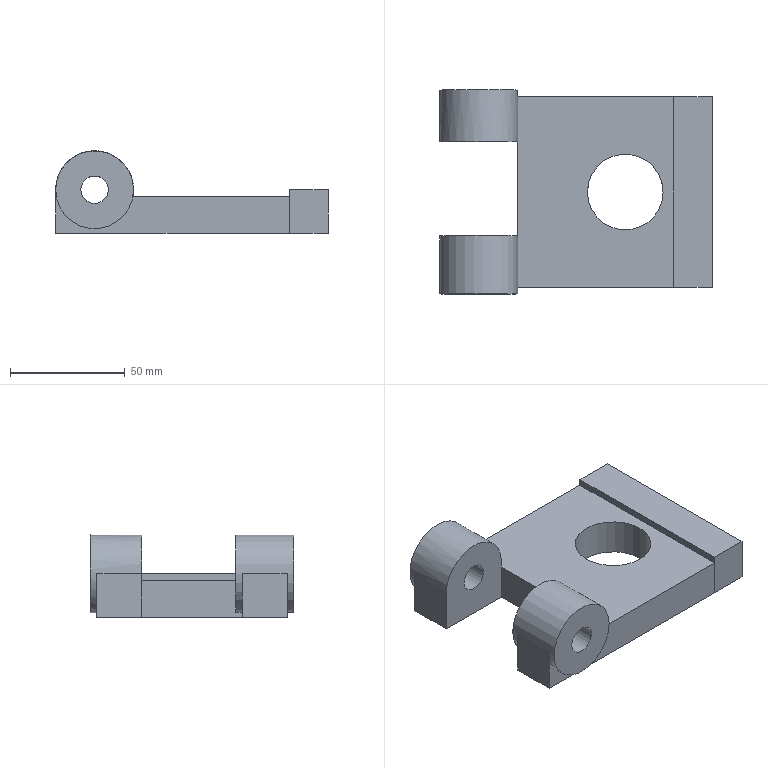Part | NX | features EXTRUDE 8, DATUM_CSYS 4, SKETCH 3, UNITE 3 | 2 solids | 26 faces | box 119 x 89 x 36 mm | volume 149069 mm3 | plane 21 | cylinder 5 | commonest cylinder face diameters 12 x2 34 x2 33 x1
STEP:
#1=CARTESIAN_POINT('',(68.,83.,0.));
#2=VERTEX_POINT('',#1);
#3=CARTESIAN_POINT('',(68.,0.,0.));
#4=VERTEX_POINT('',#3);
#5=CARTESIAN_POINT('',(68.,41.5,0.));
#6=DIRECTION('',(0.,-1.,0.));
#7=VECTOR('',#6,1000.);
#8=LINE('',#5,#7);
#9=EDGE_CURVE('',#2,#4,#8,.T.);
#10=ORIENTED_EDGE('',*,*,#9,.T.);
#11=CARTESIAN_POINT('',(68.,0.,19.));
#12=VERTEX_POINT('',#11);
#13=CARTESIAN_POINT('',(68.,0.,19.));
#14=DIRECTION('',(0.,0.,-1.));
#15=VECTOR('',#14,1000.);
#16=LINE('',#13,#15);
#17=EDGE_CURVE('',#12,#4,#16,.T.);
#18=ORIENTED_EDGE('',*,*,#17,.F.);
#19=CARTESIAN_POINT('',(68.,83.,19.));
#20=VERTEX_POINT('',#19);
#21=CARTESIAN_POINT('',(68.,83.,19.));
#22=DIRECTION('',(0.,-1.,0.));
#23=VECTOR('',#22,1000.);
#24=LINE('',#21,#23);
#25=EDGE_CURVE('',#20,#12,#24,.T.);
#26=ORIENTED_EDGE('',*,*,#25,.F.);
#27=CARTESIAN_POINT('',(68.,83.,19.));
#28=DIRECTION('',(0.,0.,-1.));
#29=VECTOR('',#28,1000.);
#30=LINE('',#27,#29);
#31=EDGE_CURVE('',#20,#2,#30,.T.);
#32=ORIENTED_EDGE('',*,*,#31,.T.);
#33=EDGE_LOOP('',(#10,#18,#26,#32));
#34=FACE_BOUND('',#33,.T.);
#35=CARTESIAN_POINT('',(68.,41.5,19.));
#36=DIRECTION('',(1.,0.,0.));
#37=DIRECTION('',(0.,1.,0.));
#38=AXIS2_PLACEMENT_3D('',#35,#36,#37);
#39=PLANE('',#38);
#40=ADVANCED_FACE('',(#34),#39,.F.);
#41=CARTESIAN_POINT('',(85.,0.,0.));
#42=VERTEX_POINT('',#41);
#43=CARTESIAN_POINT('',(68.,0.,0.));
#44=DIRECTION('',(1.,0.,0.));
#45=VECTOR('',#44,1000.);
#46=LINE('',#43,#45);
#47=EDGE_CURVE('',#4,#42,#46,.T.);
#48=ORIENTED_EDGE('',*,*,#47,.T.);
#49=CARTESIAN_POINT('',(85.,0.,19.));
#50=VERTEX_POINT('',#49);
#51=CARTESIAN_POINT('',(85.,0.,19.));
#52=DIRECTION('',(0.,0.,-1.));
#53=VECTOR('',#52,1000.);
#54=LINE('',#51,#53);
#55=EDGE_CURVE('',#50,#42,#54,.T.);
#56=ORIENTED_EDGE('',*,*,#55,.F.);
#57=CARTESIAN_POINT('',(68.,0.,19.));
#58=DIRECTION('',(1.,0.,0.));
#59=VECTOR('',#58,1000.);
#60=LINE('',#57,#59);
#61=EDGE_CURVE('',#12,#50,#60,.T.);
#62=ORIENTED_EDGE('',*,*,#61,.F.);
#63=ORIENTED_EDGE('',*,*,#17,.T.);
#64=EDGE_LOOP('',(#48,#56,#62,#63));
#65=FACE_BOUND('',#64,.T.);
#66=CARTESIAN_POINT('',(68.,0.,19.));
#67=DIRECTION('',(0.,1.,0.));
#68=DIRECTION('',(0.,0.,1.));
#69=AXIS2_PLACEMENT_3D('',#66,#67,#68);
#70=PLANE('',#69);
#71=ADVANCED_FACE('',(#65),#70,.F.);
#72=CARTESIAN_POINT('',(85.,83.,0.));
#73=VERTEX_POINT('',#72);
#74=CARTESIAN_POINT('',(85.,41.5,0.));
#75=DIRECTION('',(0.,1.,0.));
#76=VECTOR('',#75,1000.);
#77=LINE('',#74,#76);
#78=EDGE_CURVE('',#42,#73,#77,.T.);
#79=ORIENTED_EDGE('',*,*,#78,.T.);
#80=CARTESIAN_POINT('',(85.,83.,19.));
#81=VERTEX_POINT('',#80);
#82=CARTESIAN_POINT('',(85.,83.,19.));
#83=DIRECTION('',(0.,0.,-1.));
#84=VECTOR('',#83,1000.);
#85=LINE('',#82,#84);
#86=EDGE_CURVE('',#81,#73,#85,.T.);
#87=ORIENTED_EDGE('',*,*,#86,.F.);
#88=CARTESIAN_POINT('',(85.,0.,19.));
#89=DIRECTION('',(0.,1.,0.));
#90=VECTOR('',#89,1000.);
#91=LINE('',#88,#90);
#92=EDGE_CURVE('',#50,#81,#91,.T.);
#93=ORIENTED_EDGE('',*,*,#92,.F.);
#94=ORIENTED_EDGE('',*,*,#55,.T.);
#95=EDGE_LOOP('',(#79,#87,#93,#94));
#96=FACE_BOUND('',#95,.T.);
#97=CARTESIAN_POINT('',(85.,41.5,19.));
#98=DIRECTION('',(-1.,0.,0.));
#99=DIRECTION('',(0.,-1.,0.));
#100=AXIS2_PLACEMENT_3D('',#97,#98,#99);
#101=PLANE('',#100);
#102=ADVANCED_FACE('',(#96),#101,.F.);
#103=CARTESIAN_POINT('',(85.,83.,0.));
#104=DIRECTION('',(-1.,0.,0.));
#105=VECTOR('',#104,1000.);
#106=LINE('',#103,#105);
#107=EDGE_CURVE('',#73,#2,#106,.T.);
#108=ORIENTED_EDGE('',*,*,#107,.T.);
#109=ORIENTED_EDGE('',*,*,#31,.F.);
#110=CARTESIAN_POINT('',(85.,83.,19.));
#111=DIRECTION('',(-1.,0.,0.));
#112=VECTOR('',#111,1000.);
#113=LINE('',#110,#112);
#114=EDGE_CURVE('',#81,#20,#113,.T.);
#115=ORIENTED_EDGE('',*,*,#114,.F.);
#116=ORIENTED_EDGE('',*,*,#86,.T.);
#117=EDGE_LOOP('',(#108,#109,#115,#116));
#118=FACE_BOUND('',#117,.T.);
#119=CARTESIAN_POINT('',(85.,83.,19.));
#120=DIRECTION('',(0.,-1.,0.));
#121=DIRECTION('',(0.,0.,-1.));
#122=AXIS2_PLACEMENT_3D('',#119,#120,#121);
#123=PLANE('',#122);
#124=ADVANCED_FACE('',(#118),#123,.F.);
#125=ORIENTED_EDGE('',*,*,#25,.T.);
#126=ORIENTED_EDGE('',*,*,#61,.T.);
#127=ORIENTED_EDGE('',*,*,#92,.T.);
#128=ORIENTED_EDGE('',*,*,#114,.T.);
#129=EDGE_LOOP('',(#125,#126,#127,#128));
#130=FACE_BOUND('',#129,.T.);
#131=CARTESIAN_POINT('',(0.,0.,19.));
#132=DIRECTION('',(0.,0.,1.));
#133=DIRECTION('',(1.,0.,0.));
#134=AXIS2_PLACEMENT_3D('',#131,#132,#133);
#135=PLANE('',#134);
#136=ADVANCED_FACE('',(#130),#135,.T.);
#137=ORIENTED_EDGE('',*,*,#9,.F.);
#138=ORIENTED_EDGE('',*,*,#107,.F.);
#139=ORIENTED_EDGE('',*,*,#78,.F.);
#140=ORIENTED_EDGE('',*,*,#47,.F.);
#141=EDGE_LOOP('',(#137,#138,#139,#140));
#142=FACE_BOUND('',#141,.T.);
#143=CARTESIAN_POINT('',(0.,0.,0.));
#144=DIRECTION('',(0.,0.,1.));
#145=DIRECTION('',(1.,0.,0.));
#146=AXIS2_PLACEMENT_3D('',#143,#144,#145);
#147=PLANE('',#146);
#148=ADVANCED_FACE('',(#142),#147,.F.);
#149=CLOSED_SHELL('',(#40,#71,#102,#124,#136,#148));
#150=MANIFOLD_SOLID_BREP('',#149);
#151=CARTESIAN_POINT('',(-17.,86.,13.));
#152=VERTEX_POINT('',#151);
#153=CARTESIAN_POINT('',(-17.,86.,19.));
#154=DIRECTION('',(0.,-1.,0.));
#155=DIRECTION('',(0.,0.,-1.));
#156=AXIS2_PLACEMENT_3D('',#153,#154,#155);
#157=CIRCLE('',#156,6.);
#158=EDGE_CURVE('',#152,#152,#157,.T.);
#159=ORIENTED_EDGE('',*,*,#158,.F.);
#160=EDGE_LOOP('',(#159));
#161=FACE_BOUND('',#160,.T.);
#162=CARTESIAN_POINT('',(-17.,63.5,13.));
#163=VERTEX_POINT('',#162);
#164=CARTESIAN_POINT('',(-17.,63.5,19.));
#165=DIRECTION('',(0.,-1.,0.));
#166=DIRECTION('',(0.,0.,-1.));
#167=AXIS2_PLACEMENT_3D('',#164,#165,#166);
#168=CIRCLE('',#167,6.);
#169=EDGE_CURVE('',#163,#163,#168,.T.);
#170=ORIENTED_EDGE('',*,*,#169,.T.);
#171=EDGE_LOOP('',(#170));
#172=FACE_BOUND('',#171,.T.);
#173=CARTESIAN_POINT('',(-17.,86.,19.));
#174=DIRECTION('',(0.,-1.,0.));
#175=DIRECTION('',(0.,0.,-1.));
#176=AXIS2_PLACEMENT_3D('',#173,#174,#175);
#177=CYLINDRICAL_SURFACE('',#176,6.);
#178=ADVANCED_FACE('',(#161,#172),#177,.F.);
#179=CARTESIAN_POINT('',(-34.,83.,19.));
#180=VERTEX_POINT('',#179);
#181=CARTESIAN_POINT('',(-34.,63.5,19.));
#182=VERTEX_POINT('',#181);
#183=CARTESIAN_POINT('',(-34.,143.,19.));
#184=DIRECTION('',(0.,-1.,0.));
#185=VECTOR('',#184,1000.);
#186=LINE('',#183,#185);
#187=EDGE_CURVE('',#180,#182,#186,.T.);
#188=ORIENTED_EDGE('',*,*,#187,.T.);
#189=CARTESIAN_POINT('',(0.,63.5,19.));
#190=VERTEX_POINT('',#189);
#191=CARTESIAN_POINT('',(-17.,63.5,19.));
#192=DIRECTION('',(0.,-1.,0.));
#193=DIRECTION('',(0.,0.,-1.));
#194=AXIS2_PLACEMENT_3D('',#191,#192,#193);
#195=CIRCLE('',#194,17.);
#196=EDGE_CURVE('',#190,#182,#195,.T.);
#197=ORIENTED_EDGE('',*,*,#196,.F.);
#198=CARTESIAN_POINT('',(0.,83.,19.));
#199=VERTEX_POINT('',#198);
#200=CARTESIAN_POINT('',(0.,143.,19.));
#201=DIRECTION('',(0.,-1.,0.));
#202=VECTOR('',#201,1000.);
#203=LINE('',#200,#202);
#204=EDGE_CURVE('',#199,#190,#203,.T.);
#205=ORIENTED_EDGE('',*,*,#204,.F.);
#206=CARTESIAN_POINT('',(-17.,83.,19.));
#207=DIRECTION('',(0.,-1.,0.));
#208=DIRECTION('',(1.,0.,0.));
#209=AXIS2_PLACEMENT_3D('',#206,#207,#208);
#210=CIRCLE('',#209,17.);
#211=EDGE_CURVE('',#180,#199,#210,.T.);
#212=ORIENTED_EDGE('',*,*,#211,.F.);
#213=EDGE_LOOP('',(#188,#197,#205,#212));
#214=FACE_BOUND('',#213,.T.);
#215=CARTESIAN_POINT('',(-17.,86.,2.));
#216=VERTEX_POINT('',#215);
#217=CARTESIAN_POINT('',(-17.,86.,19.));
#218=DIRECTION('',(0.,-1.,0.));
#219=DIRECTION('',(0.,0.,-1.));
#220=AXIS2_PLACEMENT_3D('',#217,#218,#219);
#221=CIRCLE('',#220,17.);
#222=EDGE_CURVE('',#216,#216,#221,.T.);
#223=ORIENTED_EDGE('',*,*,#222,.T.);
#224=EDGE_LOOP('',(#223));
#225=FACE_BOUND('',#224,.T.);
#226=CARTESIAN_POINT('',(-17.,86.,19.));
#227=DIRECTION('',(0.,-1.,0.));
#228=DIRECTION('',(0.,0.,-1.));
#229=AXIS2_PLACEMENT_3D('',#226,#227,#228);
#230=CYLINDRICAL_SURFACE('',#229,17.);
#231=ADVANCED_FACE('',(#214,#225),#230,.T.);
#232=ORIENTED_EDGE('',*,*,#222,.F.);
#233=EDGE_LOOP('',(#232));
#234=FACE_BOUND('',#233,.T.);
#235=ORIENTED_EDGE('',*,*,#158,.T.);
#236=EDGE_LOOP('',(#235));
#237=FACE_BOUND('',#236,.T.);
#238=CARTESIAN_POINT('',(-17.,86.,19.));
#239=DIRECTION('',(0.,-1.,0.));
#240=DIRECTION('',(0.,0.,-1.));
#241=AXIS2_PLACEMENT_3D('',#238,#239,#240);
#242=PLANE('',#241);
#243=ADVANCED_FACE('',(#234,#237),#242,.F.);
#244=ORIENTED_EDGE('',*,*,#169,.F.);
#245=EDGE_LOOP('',(#244));
#246=FACE_BOUND('',#245,.T.);
#247=ORIENTED_EDGE('',*,*,#196,.T.);
#248=CARTESIAN_POINT('',(-34.,63.5,0.));
#249=VERTEX_POINT('',#248);
#250=CARTESIAN_POINT('',(-34.,63.5,25.));
#251=DIRECTION('',(0.,0.,-1.));
#252=VECTOR('',#251,1000.);
#253=LINE('',#250,#252);
#254=EDGE_CURVE('',#182,#249,#253,.T.);
#255=ORIENTED_EDGE('',*,*,#254,.T.);
#256=CARTESIAN_POINT('',(0.,63.5,0.));
#257=VERTEX_POINT('',#256);
#258=CARTESIAN_POINT('',(-34.,63.5,0.));
#259=DIRECTION('',(1.,0.,0.));
#260=VECTOR('',#259,1000.);
#261=LINE('',#258,#260);
#262=EDGE_CURVE('',#249,#257,#261,.T.);
#263=ORIENTED_EDGE('',*,*,#262,.T.);
#264=CARTESIAN_POINT('',(0.,63.5,16.));
#265=VERTEX_POINT('',#264);
#266=CARTESIAN_POINT('',(0.,63.5,25.));
#267=DIRECTION('',(0.,0.,-1.));
#268=VECTOR('',#267,1000.);
#269=LINE('',#266,#268);
#270=EDGE_CURVE('',#265,#257,#269,.T.);
#271=ORIENTED_EDGE('',*,*,#270,.F.);
#272=CARTESIAN_POINT('',(0.,63.5,25.));
#273=DIRECTION('',(0.,0.,-1.));
#274=VECTOR('',#273,1000.);
#275=LINE('',#272,#274);
#276=EDGE_CURVE('',#190,#265,#275,.T.);
#277=ORIENTED_EDGE('',*,*,#276,.F.);
#278=EDGE_LOOP('',(#247,#255,#263,#271,#277));
#279=FACE_BOUND('',#278,.T.);
#280=CARTESIAN_POINT('',(-17.,63.5,19.));
#281=DIRECTION('',(0.,-1.,0.));
#282=DIRECTION('',(0.,0.,-1.));
#283=AXIS2_PLACEMENT_3D('',#280,#281,#282);
#284=PLANE('',#283);
#285=ADVANCED_FACE('',(#246,#279),#284,.T.);
#286=CARTESIAN_POINT('',(-34.,19.5,19.));
#287=VERTEX_POINT('',#286);
#288=CARTESIAN_POINT('',(-34.,19.5,0.));
#289=VERTEX_POINT('',#288);
#290=CARTESIAN_POINT('',(-34.,19.5,25.));
#291=DIRECTION('',(0.,0.,-1.));
#292=VECTOR('',#291,1000.);
#293=LINE('',#290,#292);
#294=EDGE_CURVE('',#287,#289,#293,.T.);
#295=ORIENTED_EDGE('',*,*,#294,.F.);
#296=CARTESIAN_POINT('',(0.,19.5,19.));
#297=VERTEX_POINT('',#296);
#298=CARTESIAN_POINT('',(-17.,19.5,19.));
#299=DIRECTION('',(0.,-1.,0.));
#300=DIRECTION('',(1.,0.,0.));
#301=AXIS2_PLACEMENT_3D('',#298,#299,#300);
#302=CIRCLE('',#301,17.);
#303=EDGE_CURVE('',#287,#297,#302,.T.);
#304=ORIENTED_EDGE('',*,*,#303,.T.);
#305=CARTESIAN_POINT('',(0.,19.5,16.));
#306=VERTEX_POINT('',#305);
#307=CARTESIAN_POINT('',(0.,19.5,25.));
#308=DIRECTION('',(0.,0.,-1.));
#309=VECTOR('',#308,1000.);
#310=LINE('',#307,#309);
#311=EDGE_CURVE('',#297,#306,#310,.T.);
#312=ORIENTED_EDGE('',*,*,#311,.T.);
#313=CARTESIAN_POINT('',(0.,19.5,0.));
#314=VERTEX_POINT('',#313);
#315=CARTESIAN_POINT('',(0.,19.5,25.));
#316=DIRECTION('',(0.,0.,-1.));
#317=VECTOR('',#316,1000.);
#318=LINE('',#315,#317);
#319=EDGE_CURVE('',#306,#314,#318,.T.);
#320=ORIENTED_EDGE('',*,*,#319,.T.);
#321=CARTESIAN_POINT('',(0.,19.5,0.));
#322=DIRECTION('',(-1.,0.,0.));
#323=VECTOR('',#322,1000.);
#324=LINE('',#321,#323);
#325=EDGE_CURVE('',#314,#289,#324,.T.);
#326=ORIENTED_EDGE('',*,*,#325,.T.);
#327=EDGE_LOOP('',(#295,#304,#312,#320,#326));
#328=FACE_BOUND('',#327,.T.);
#329=CARTESIAN_POINT('',(0.,19.5,25.));
#330=DIRECTION('',(0.,-1.,0.));
#331=DIRECTION('',(1.,0.,0.));
#332=AXIS2_PLACEMENT_3D('',#329,#330,#331);
#333=PLANE('',#332);
#334=ADVANCED_FACE('',(#328),#333,.F.);
#335=CARTESIAN_POINT('',(0.,0.,19.));
#336=VERTEX_POINT('',#335);
#337=CARTESIAN_POINT('',(0.,0.,16.));
#338=VERTEX_POINT('',#337);
#339=CARTESIAN_POINT('',(0.,0.,25.));
#340=DIRECTION('',(0.,0.,-1.));
#341=VECTOR('',#340,1000.);
#342=LINE('',#339,#341);
#343=EDGE_CURVE('',#336,#338,#342,.T.);
#344=ORIENTED_EDGE('',*,*,#343,.F.);
#345=CARTESIAN_POINT('',(-34.,0.,19.));
#346=VERTEX_POINT('',#345);
#347=CARTESIAN_POINT('',(-17.,0.,19.));
#348=DIRECTION('',(0.,1.,0.));
#349=DIRECTION('',(-1.,0.,0.));
#350=AXIS2_PLACEMENT_3D('',#347,#348,#349);
#351=CIRCLE('',#350,17.);
#352=EDGE_CURVE('',#346,#336,#351,.F.);
#353=ORIENTED_EDGE('',*,*,#352,.F.);
#354=CARTESIAN_POINT('',(-34.,0.,0.));
#355=VERTEX_POINT('',#354);
#356=CARTESIAN_POINT('',(-34.,0.,25.));
#357=DIRECTION('',(0.,0.,-1.));
#358=VECTOR('',#357,1000.);
#359=LINE('',#356,#358);
#360=EDGE_CURVE('',#346,#355,#359,.T.);
#361=ORIENTED_EDGE('',*,*,#360,.T.);
#362=CARTESIAN_POINT('',(68.,0.,0.));
#363=VERTEX_POINT('',#362);
#364=CARTESIAN_POINT('',(-34.,0.,0.));
#365=DIRECTION('',(1.,0.,0.));
#366=VECTOR('',#365,1000.);
#367=LINE('',#364,#366);
#368=EDGE_CURVE('',#355,#363,#367,.T.);
#369=ORIENTED_EDGE('',*,*,#368,.T.);
#370=CARTESIAN_POINT('',(68.,0.,16.));
#371=VERTEX_POINT('',#370);
#372=CARTESIAN_POINT('',(68.,0.,16.));
#373=DIRECTION('',(0.,0.,-1.));
#374=VECTOR('',#373,1000.);
#375=LINE('',#372,#374);
#376=EDGE_CURVE('',#371,#363,#375,.T.);
#377=ORIENTED_EDGE('',*,*,#376,.F.);
#378=CARTESIAN_POINT('',(0.,0.,16.));
#379=DIRECTION('',(1.,0.,0.));
#380=VECTOR('',#379,1000.);
#381=LINE('',#378,#380);
#382=EDGE_CURVE('',#338,#371,#381,.T.);
#383=ORIENTED_EDGE('',*,*,#382,.F.);
#384=EDGE_LOOP('',(#344,#353,#361,#369,#377,#383));
#385=FACE_BOUND('',#384,.T.);
#386=CARTESIAN_POINT('',(-34.,0.,25.));
#387=DIRECTION('',(0.,1.,0.));
#388=DIRECTION('',(-1.,0.,0.));
#389=AXIS2_PLACEMENT_3D('',#386,#387,#388);
#390=PLANE('',#389);
#391=ADVANCED_FACE('',(#385),#390,.F.);
#392=ORIENTED_EDGE('',*,*,#187,.F.);
#393=CARTESIAN_POINT('',(-34.,83.,0.));
#394=VERTEX_POINT('',#393);
#395=CARTESIAN_POINT('',(-34.,83.,25.));
#396=DIRECTION('',(0.,0.,-1.));
#397=VECTOR('',#396,1000.);
#398=LINE('',#395,#397);
#399=EDGE_CURVE('',#180,#394,#398,.T.);
#400=ORIENTED_EDGE('',*,*,#399,.T.);
#401=CARTESIAN_POINT('',(-34.,83.,0.));
#402=DIRECTION('',(0.,-1.,0.));
#403=VECTOR('',#402,1000.);
#404=LINE('',#401,#403);
#405=EDGE_CURVE('',#394,#249,#404,.T.);
#406=ORIENTED_EDGE('',*,*,#405,.T.);
#407=ORIENTED_EDGE('',*,*,#254,.F.);
#408=EDGE_LOOP('',(#392,#400,#406,#407));
#409=FACE_BOUND('',#408,.T.);
#410=CARTESIAN_POINT('',(-34.,83.,25.));
#411=DIRECTION('',(1.,0.,0.));
#412=DIRECTION('',(0.,0.,-1.));
#413=AXIS2_PLACEMENT_3D('',#410,#411,#412);
#414=PLANE('',#413);
#415=ADVANCED_FACE('',(#409),#414,.F.);
#416=CARTESIAN_POINT('',(-34.,143.,19.));
#417=DIRECTION('',(0.,-1.,0.));
#418=VECTOR('',#417,1000.);
#419=LINE('',#416,#418);
#420=EDGE_CURVE('',#287,#346,#419,.T.);
#421=ORIENTED_EDGE('',*,*,#420,.F.);
#422=ORIENTED_EDGE('',*,*,#294,.T.);
#423=CARTESIAN_POINT('',(-34.,19.5,0.));
#424=DIRECTION('',(0.,-1.,0.));
#425=VECTOR('',#424,1000.);
#426=LINE('',#423,#425);
#427=EDGE_CURVE('',#289,#355,#426,.T.);
#428=ORIENTED_EDGE('',*,*,#427,.T.);
#429=ORIENTED_EDGE('',*,*,#360,.F.);
#430=EDGE_LOOP('',(#421,#422,#428,#429));
#431=FACE_BOUND('',#430,.T.);
#432=CARTESIAN_POINT('',(-34.,19.5,25.));
#433=DIRECTION('',(1.,0.,0.));
#434=DIRECTION('',(0.,0.,-1.));
#435=AXIS2_PLACEMENT_3D('',#432,#433,#434);
#436=PLANE('',#435);
#437=ADVANCED_FACE('',(#431),#436,.F.);
#438=CARTESIAN_POINT('',(0.,83.,16.));
#439=VERTEX_POINT('',#438);
#440=CARTESIAN_POINT('',(0.,83.,25.));
#441=DIRECTION('',(0.,0.,-1.));
#442=VECTOR('',#441,1000.);
#443=LINE('',#440,#442);
#444=EDGE_CURVE('',#199,#439,#443,.T.);
#445=ORIENTED_EDGE('',*,*,#444,.F.);
#446=ORIENTED_EDGE('',*,*,#204,.T.);
#447=ORIENTED_EDGE('',*,*,#276,.T.);
#448=CARTESIAN_POINT('',(0.,83.,16.));
#449=DIRECTION('',(0.,-1.,0.));
#450=VECTOR('',#449,1000.);
#451=LINE('',#448,#450);
#452=EDGE_CURVE('',#439,#265,#451,.T.);
#453=ORIENTED_EDGE('',*,*,#452,.F.);
#454=EDGE_LOOP('',(#445,#446,#447,#453));
#455=FACE_BOUND('',#454,.T.);
#456=CARTESIAN_POINT('',(0.,63.5,25.));
#457=DIRECTION('',(-1.,0.,0.));
#458=DIRECTION('',(0.,0.,1.));
#459=AXIS2_PLACEMENT_3D('',#456,#457,#458);
#460=PLANE('',#459);
#461=ADVANCED_FACE('',(#455),#460,.F.);
#462=ORIENTED_EDGE('',*,*,#211,.T.);
#463=ORIENTED_EDGE('',*,*,#444,.T.);
#464=CARTESIAN_POINT('',(68.,83.,16.));
#465=VERTEX_POINT('',#464);
#466=CARTESIAN_POINT('',(68.,83.,16.));
#467=DIRECTION('',(-1.,0.,0.));
#468=VECTOR('',#467,1000.);
#469=LINE('',#466,#468);
#470=EDGE_CURVE('',#465,#439,#469,.T.);
#471=ORIENTED_EDGE('',*,*,#470,.F.);
#472=CARTESIAN_POINT('',(68.,83.,0.));
#473=VERTEX_POINT('',#472);
#474=CARTESIAN_POINT('',(68.,83.,16.));
#475=DIRECTION('',(0.,0.,-1.));
#476=VECTOR('',#475,1000.);
#477=LINE('',#474,#476);
#478=EDGE_CURVE('',#465,#473,#477,.T.);
#479=ORIENTED_EDGE('',*,*,#478,.T.);
#480=CARTESIAN_POINT('',(0.,83.,0.));
#481=DIRECTION('',(-1.,0.,0.));
#482=VECTOR('',#481,1000.);
#483=LINE('',#480,#482);
#484=EDGE_CURVE('',#473,#394,#483,.T.);
#485=ORIENTED_EDGE('',*,*,#484,.T.);
#486=ORIENTED_EDGE('',*,*,#399,.F.);
#487=EDGE_LOOP('',(#462,#463,#471,#479,#485,#486));
#488=FACE_BOUND('',#487,.T.);
#489=CARTESIAN_POINT('',(0.,83.,25.));
#490=DIRECTION('',(0.,-1.,0.));
#491=DIRECTION('',(1.,0.,0.));
#492=AXIS2_PLACEMENT_3D('',#489,#490,#491);
#493=PLANE('',#492);
#494=ADVANCED_FACE('',(#488),#493,.F.);
#495=ORIENTED_EDGE('',*,*,#405,.F.);
#496=ORIENTED_EDGE('',*,*,#484,.F.);
#497=CARTESIAN_POINT('',(68.,41.5,0.));
#498=DIRECTION('',(0.,1.,0.));
#499=VECTOR('',#498,1000.);
#500=LINE('',#497,#499);
#501=EDGE_CURVE('',#363,#473,#500,.T.);
#502=ORIENTED_EDGE('',*,*,#501,.F.);
#503=ORIENTED_EDGE('',*,*,#368,.F.);
#504=ORIENTED_EDGE('',*,*,#427,.F.);
#505=ORIENTED_EDGE('',*,*,#325,.F.);
#506=CARTESIAN_POINT('',(0.,41.5,0.));
#507=DIRECTION('',(0.,-1.,0.));
#508=VECTOR('',#507,1000.);
#509=LINE('',#506,#508);
#510=EDGE_CURVE('',#257,#314,#509,.T.);
#511=ORIENTED_EDGE('',*,*,#510,.F.);
#512=ORIENTED_EDGE('',*,*,#262,.F.);
#513=EDGE_LOOP('',(#495,#496,#502,#503,#504,#505,#511,#512));
#514=FACE_BOUND('',#513,.T.);
#515=CARTESIAN_POINT('',(63.5,41.5,0.));
#516=VERTEX_POINT('',#515);
#517=CARTESIAN_POINT('',(47.,41.5,0.));
#518=DIRECTION('',(0.,0.,-1.));
#519=DIRECTION('',(1.,0.,0.));
#520=AXIS2_PLACEMENT_3D('',#517,#518,#519);
#521=CIRCLE('',#520,16.5);
#522=EDGE_CURVE('',#516,#516,#521,.T.);
#523=ORIENTED_EDGE('',*,*,#522,.F.);
#524=EDGE_LOOP('',(#523));
#525=FACE_BOUND('',#524,.T.);
#526=CARTESIAN_POINT('',(0.,0.,0.));
#527=DIRECTION('',(0.,0.,1.));
#528=DIRECTION('',(1.,0.,0.));
#529=AXIS2_PLACEMENT_3D('',#526,#527,#528);
#530=PLANE('',#529);
#531=ADVANCED_FACE('',(#514,#525),#530,.F.);
#532=CARTESIAN_POINT('',(0.,83.,16.));
#533=DIRECTION('',(0.,-1.,0.));
#534=VECTOR('',#533,1000.);
#535=LINE('',#532,#534);
#536=EDGE_CURVE('',#265,#306,#535,.T.);
#537=ORIENTED_EDGE('',*,*,#536,.F.);
#538=ORIENTED_EDGE('',*,*,#270,.T.);
#539=ORIENTED_EDGE('',*,*,#510,.T.);
#540=ORIENTED_EDGE('',*,*,#319,.F.);
#541=EDGE_LOOP('',(#537,#538,#539,#540));
#542=FACE_BOUND('',#541,.T.);
#543=CARTESIAN_POINT('',(0.,41.5,16.));
#544=DIRECTION('',(1.,0.,0.));
#545=DIRECTION('',(0.,0.,-1.));
#546=AXIS2_PLACEMENT_3D('',#543,#544,#545);
#547=PLANE('',#546);
#548=ADVANCED_FACE('',(#542),#547,.F.);
#549=ORIENTED_EDGE('',*,*,#311,.F.);
#550=CARTESIAN_POINT('',(0.,143.,19.));
#551=DIRECTION('',(0.,-1.,0.));
#552=VECTOR('',#551,1000.);
#553=LINE('',#550,#552);
#554=EDGE_CURVE('',#297,#336,#553,.T.);
#555=ORIENTED_EDGE('',*,*,#554,.T.);
#556=ORIENTED_EDGE('',*,*,#343,.T.);
#557=CARTESIAN_POINT('',(0.,83.,16.));
#558=DIRECTION('',(0.,-1.,0.));
#559=VECTOR('',#558,1000.);
#560=LINE('',#557,#559);
#561=EDGE_CURVE('',#306,#338,#560,.T.);
#562=ORIENTED_EDGE('',*,*,#561,.F.);
#563=EDGE_LOOP('',(#549,#555,#556,#562));
#564=FACE_BOUND('',#563,.T.);
#565=CARTESIAN_POINT('',(0.,0.,25.));
#566=DIRECTION('',(-1.,0.,0.));
#567=DIRECTION('',(0.,0.,1.));
#568=AXIS2_PLACEMENT_3D('',#565,#566,#567);
#569=PLANE('',#568);
#570=ADVANCED_FACE('',(#564),#569,.F.);
#571=ORIENTED_EDGE('',*,*,#501,.T.);
#572=ORIENTED_EDGE('',*,*,#478,.F.);
#573=CARTESIAN_POINT('',(68.,0.,16.));
#574=DIRECTION('',(0.,1.,0.));
#575=VECTOR('',#574,1000.);
#576=LINE('',#573,#575);
#577=EDGE_CURVE('',#371,#465,#576,.T.);
#578=ORIENTED_EDGE('',*,*,#577,.F.);
#579=ORIENTED_EDGE('',*,*,#376,.T.);
#580=EDGE_LOOP('',(#571,#572,#578,#579));
#581=FACE_BOUND('',#580,.T.);
#582=CARTESIAN_POINT('',(68.,41.5,16.));
#583=DIRECTION('',(-1.,0.,0.));
#584=DIRECTION('',(0.,-1.,0.));
#585=AXIS2_PLACEMENT_3D('',#582,#583,#584);
#586=PLANE('',#585);
#587=ADVANCED_FACE('',(#581),#586,.F.);
#588=ORIENTED_EDGE('',*,*,#522,.T.);
#589=EDGE_LOOP('',(#588));
#590=FACE_BOUND('',#589,.T.);
#591=CARTESIAN_POINT('',(63.5,41.5,16.));
#592=VERTEX_POINT('',#591);
#593=CARTESIAN_POINT('',(47.,41.5,16.));
#594=DIRECTION('',(0.,0.,-1.));
#595=DIRECTION('',(1.,0.,0.));
#596=AXIS2_PLACEMENT_3D('',#593,#594,#595);
#597=CIRCLE('',#596,16.5);
#598=EDGE_CURVE('',#592,#592,#597,.T.);
#599=ORIENTED_EDGE('',*,*,#598,.F.);
#600=EDGE_LOOP('',(#599));
#601=FACE_BOUND('',#600,.T.);
#602=CARTESIAN_POINT('',(47.,41.5,16.));
#603=DIRECTION('',(0.,0.,-1.));
#604=DIRECTION('',(-1.,0.,0.));
#605=AXIS2_PLACEMENT_3D('',#602,#603,#604);
#606=CYLINDRICAL_SURFACE('',#605,16.5);
#607=ADVANCED_FACE('',(#590,#601),#606,.F.);
#608=ORIENTED_EDGE('',*,*,#452,.T.);
#609=ORIENTED_EDGE('',*,*,#536,.T.);
#610=ORIENTED_EDGE('',*,*,#561,.T.);
#611=ORIENTED_EDGE('',*,*,#382,.T.);
#612=ORIENTED_EDGE('',*,*,#577,.T.);
#613=ORIENTED_EDGE('',*,*,#470,.T.);
#614=EDGE_LOOP('',(#608,#609,#610,#611,#612,#613));
#615=FACE_BOUND('',#614,.T.);
#616=ORIENTED_EDGE('',*,*,#598,.T.);
#617=EDGE_LOOP('',(#616));
#618=FACE_BOUND('',#617,.T.);
#619=CARTESIAN_POINT('',(47.,41.5,16.));
#620=DIRECTION('',(0.,0.,-1.));
#621=DIRECTION('',(-1.,0.,0.));
#622=AXIS2_PLACEMENT_3D('',#619,#620,#621);
#623=PLANE('',#622);
#624=ADVANCED_FACE('',(#615,#618),#623,.F.);
#625=ORIENTED_EDGE('',*,*,#554,.F.);
#626=ORIENTED_EDGE('',*,*,#303,.F.);
#627=ORIENTED_EDGE('',*,*,#420,.T.);
#628=ORIENTED_EDGE('',*,*,#352,.T.);
#629=EDGE_LOOP('',(#625,#626,#627,#628));
#630=FACE_BOUND('',#629,.T.);
#631=CARTESIAN_POINT('',(0.,-3.,19.));
#632=VERTEX_POINT('',#631);
#633=CARTESIAN_POINT('',(-17.,-3.,19.));
#634=DIRECTION('',(0.,-1.,0.));
#635=DIRECTION('',(1.,0.,0.));
#636=AXIS2_PLACEMENT_3D('',#633,#634,#635);
#637=CIRCLE('',#636,17.);
#638=EDGE_CURVE('',#632,#632,#637,.F.);
#639=ORIENTED_EDGE('',*,*,#638,.T.);
#640=EDGE_LOOP('',(#639));
#641=FACE_BOUND('',#640,.T.);
#642=CARTESIAN_POINT('',(0.,22.5,19.));
#643=VERTEX_POINT('',#642);
#644=CARTESIAN_POINT('',(-17.,22.5,19.));
#645=DIRECTION('',(0.,-1.,0.));
#646=DIRECTION('',(1.,0.,0.));
#647=AXIS2_PLACEMENT_3D('',#644,#645,#646);
#648=CIRCLE('',#647,17.);
#649=EDGE_CURVE('',#643,#643,#648,.F.);
#650=ORIENTED_EDGE('',*,*,#649,.F.);
#651=EDGE_LOOP('',(#650));
#652=FACE_BOUND('',#651,.T.);
#653=CARTESIAN_POINT('',(-17.,143.,19.));
#654=DIRECTION('',(0.,-1.,0.));
#655=DIRECTION('',(0.,0.,-1.));
#656=AXIS2_PLACEMENT_3D('',#653,#654,#655);
#657=CYLINDRICAL_SURFACE('',#656,17.);
#658=ADVANCED_FACE('',(#630,#641,#652),#657,.T.);
#659=CARTESIAN_POINT('',(-11.,22.5,19.));
#660=VERTEX_POINT('',#659);
#661=CARTESIAN_POINT('',(-17.,22.5,19.));
#662=DIRECTION('',(0.,1.,0.));
#663=DIRECTION('',(1.,0.,0.));
#664=AXIS2_PLACEMENT_3D('',#661,#662,#663);
#665=CIRCLE('',#664,6.);
#666=EDGE_CURVE('',#660,#660,#665,.F.);
#667=ORIENTED_EDGE('',*,*,#666,.F.);
#668=EDGE_LOOP('',(#667));
#669=FACE_BOUND('',#668,.T.);
#670=CARTESIAN_POINT('',(-11.,-3.,19.));
#671=VERTEX_POINT('',#670);
#672=CARTESIAN_POINT('',(-17.,-3.,19.));
#673=DIRECTION('',(0.,1.,0.));
#674=DIRECTION('',(1.,0.,0.));
#675=AXIS2_PLACEMENT_3D('',#672,#673,#674);
#676=CIRCLE('',#675,6.);
#677=EDGE_CURVE('',#671,#671,#676,.F.);
#678=ORIENTED_EDGE('',*,*,#677,.T.);
#679=EDGE_LOOP('',(#678));
#680=FACE_BOUND('',#679,.T.);
#681=CARTESIAN_POINT('',(-17.,22.5,19.));
#682=DIRECTION('',(0.,-1.,0.));
#683=DIRECTION('',(0.,0.,-1.));
#684=AXIS2_PLACEMENT_3D('',#681,#682,#683);
#685=CYLINDRICAL_SURFACE('',#684,6.);
#686=ADVANCED_FACE('',(#669,#680),#685,.F.);
#687=ORIENTED_EDGE('',*,*,#649,.T.);
#688=EDGE_LOOP('',(#687));
#689=FACE_BOUND('',#688,.T.);
#690=ORIENTED_EDGE('',*,*,#666,.T.);
#691=EDGE_LOOP('',(#690));
#692=FACE_BOUND('',#691,.T.);
#693=CARTESIAN_POINT('',(-17.,22.5,19.));
#694=DIRECTION('',(0.,-1.,0.));
#695=DIRECTION('',(0.,0.,-1.));
#696=AXIS2_PLACEMENT_3D('',#693,#694,#695);
#697=PLANE('',#696);
#698=ADVANCED_FACE('',(#689,#692),#697,.F.);
#699=ORIENTED_EDGE('',*,*,#638,.F.);
#700=EDGE_LOOP('',(#699));
#701=FACE_BOUND('',#700,.T.);
#702=ORIENTED_EDGE('',*,*,#677,.F.);
#703=EDGE_LOOP('',(#702));
#704=FACE_BOUND('',#703,.T.);
#705=CARTESIAN_POINT('',(-17.,-3.,19.));
#706=DIRECTION('',(0.,-1.,0.));
#707=DIRECTION('',(0.,0.,-1.));
#708=AXIS2_PLACEMENT_3D('',#705,#706,#707);
#709=PLANE('',#708);
#710=ADVANCED_FACE('',(#701,#704),#709,.T.);
#711=CLOSED_SHELL('',(#178,#231,#243,#285,#334,#391,#415,#437,#461,#494,#531,#548,#570,#587,#607,#624,#658,#686,#698,#710));
#712=MANIFOLD_SOLID_BREP('',#711);
#713=(LENGTH_UNIT()NAMED_UNIT(*)SI_UNIT(.MILLI.,.METRE.));
#714=UNCERTAINTY_MEASURE_WITH_UNIT(LENGTH_MEASURE(0.00001),#713,'','');
#715=(NAMED_UNIT(*)PLANE_ANGLE_UNIT()SI_UNIT($,.RADIAN.));
#716=(NAMED_UNIT(*)SI_UNIT($,.STERADIAN.)SOLID_ANGLE_UNIT());
#717=(GEOMETRIC_REPRESENTATION_CONTEXT(3)GLOBAL_UNCERTAINTY_ASSIGNED_CONTEXT((#714))GLOBAL_UNIT_ASSIGNED_CONTEXT((#713,#715,#716))REPRESENTATION_CONTEXT('',''));
#718=ADVANCED_BREP_SHAPE_REPRESENTATION('',(#150,#712),#717);